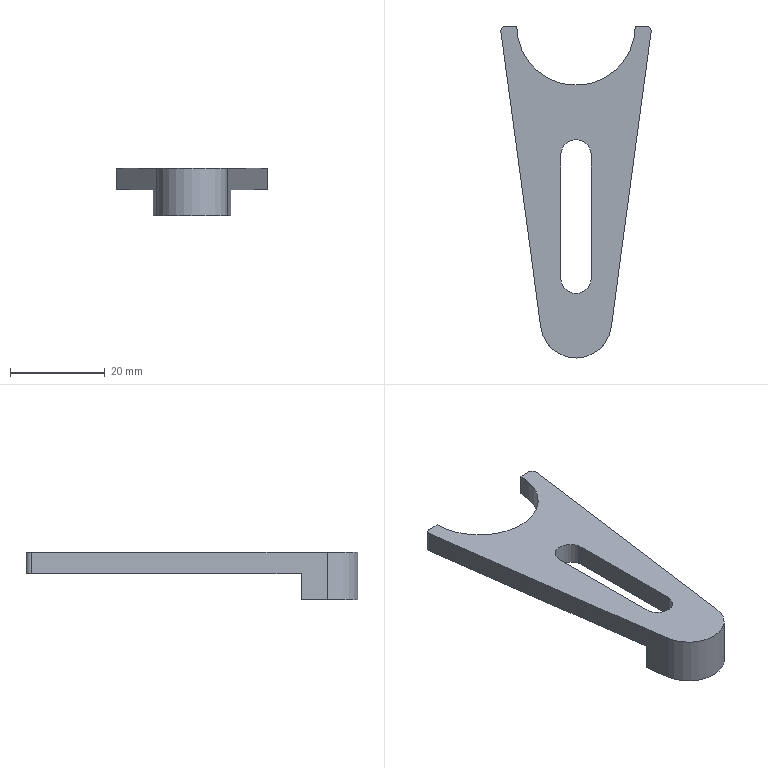Part | STEP file | 1358D2-4.stp.STEP | 1 solid | 16 faces | box 31.712 x 70 x 10 mm | volume 5901 mm3 | plane 10 | cylinder 6 | commonest cylinder face diameters 2 x2 6.4 x2 15 x1 25 x1
STEP:
#1=CARTESIAN_POINT('',(8.175,-23.,0.));
#2=VERTEX_POINT('',#1);
#3=CARTESIAN_POINT('',(7.433,-28.503,0.));
#4=VERTEX_POINT('',#3);
#5=CARTESIAN_POINT('',(8.175,-23.,0.));
#6=DIRECTION('',(-0.1337,-0.991,0.));
#7=VECTOR('',#6,1000.);
#8=LINE('',#5,#7);
#9=EDGE_CURVE('',#2,#4,#8,.T.);
#10=ORIENTED_EDGE('',*,*,#9,.T.);
#11=CARTESIAN_POINT('',(-7.433,-28.503,0.));
#12=VERTEX_POINT('',#11);
#13=CARTESIAN_POINT('',(0.,-27.5,0.));
#14=DIRECTION('',(0.,0.,1.));
#15=DIRECTION('',(-0.991,-0.1337,0.));
#16=AXIS2_PLACEMENT_3D('',#13,#14,#15);
#17=CIRCLE('',#16,7.5);
#18=EDGE_CURVE('',#12,#4,#17,.T.);
#19=ORIENTED_EDGE('',*,*,#18,.F.);
#20=CARTESIAN_POINT('',(-8.175,-23.,0.));
#21=VERTEX_POINT('',#20);
#22=CARTESIAN_POINT('',(-7.433,-28.503,0.));
#23=DIRECTION('',(-0.1337,0.991,0.));
#24=VECTOR('',#23,1000.);
#25=LINE('',#22,#24);
#26=EDGE_CURVE('',#12,#21,#25,.T.);
#27=ORIENTED_EDGE('',*,*,#26,.T.);
#28=CARTESIAN_POINT('',(-8.175,-23.,0.));
#29=DIRECTION('',(1.,0.,0.));
#30=VECTOR('',#29,1000.);
#31=LINE('',#28,#30);
#32=EDGE_CURVE('',#21,#2,#31,.T.);
#33=ORIENTED_EDGE('',*,*,#32,.T.);
#34=EDGE_LOOP('',(#10,#19,#27,#33));
#35=FACE_OUTER_BOUND('',#34,.T.);
#36=CARTESIAN_POINT('',(0.,0.,0.));
#37=DIRECTION('',(0.,0.,1.));
#38=DIRECTION('',(1.,0.,0.));
#39=AXIS2_PLACEMENT_3D('',#36,#37,#38);
#40=PLANE('',#39);
#41=ADVANCED_FACE('',(#35),#40,.F.);
#42=CARTESIAN_POINT('',(-8.175,-23.,5.5));
#43=VERTEX_POINT('',#42);
#44=CARTESIAN_POINT('',(-8.175,-23.,0.));
#45=DIRECTION('',(0.,0.,1.));
#46=VECTOR('',#45,1000.);
#47=LINE('',#44,#46);
#48=EDGE_CURVE('',#21,#43,#47,.T.);
#49=ORIENTED_EDGE('',*,*,#48,.T.);
#50=CARTESIAN_POINT('',(8.175,-23.,5.5));
#51=VERTEX_POINT('',#50);
#52=CARTESIAN_POINT('',(8.175,-23.,5.5));
#53=DIRECTION('',(-1.,0.,0.));
#54=VECTOR('',#53,1000.);
#55=LINE('',#52,#54);
#56=EDGE_CURVE('',#51,#43,#55,.T.);
#57=ORIENTED_EDGE('',*,*,#56,.F.);
#58=CARTESIAN_POINT('',(8.175,-23.,0.));
#59=DIRECTION('',(0.,0.,1.));
#60=VECTOR('',#59,1000.);
#61=LINE('',#58,#60);
#62=EDGE_CURVE('',#2,#51,#61,.T.);
#63=ORIENTED_EDGE('',*,*,#62,.F.);
#64=ORIENTED_EDGE('',*,*,#32,.F.);
#65=EDGE_LOOP('',(#49,#57,#63,#64));
#66=FACE_OUTER_BOUND('',#65,.T.);
#67=CARTESIAN_POINT('',(30.,-23.,0.));
#68=DIRECTION('',(0.,-1.,0.));
#69=DIRECTION('',(0.,0.,-1.));
#70=AXIS2_PLACEMENT_3D('',#67,#68,#69);
#71=PLANE('',#70);
#72=ADVANCED_FACE('',(#66),#71,.F.);
#73=CARTESIAN_POINT('',(15.847,33.866,10.));
#74=VERTEX_POINT('',#73);
#75=CARTESIAN_POINT('',(7.433,-28.503,10.));
#76=VERTEX_POINT('',#75);
#77=CARTESIAN_POINT('',(15.847,33.866,10.));
#78=DIRECTION('',(-0.1337,-0.991,0.));
#79=VECTOR('',#78,1000.);
#80=LINE('',#77,#79);
#81=EDGE_CURVE('',#74,#76,#80,.T.);
#82=ORIENTED_EDGE('',*,*,#81,.T.);
#83=CARTESIAN_POINT('',(7.433,-28.503,10.));
#84=DIRECTION('',(0.,0.,-1.));
#85=VECTOR('',#84,1000.);
#86=LINE('',#83,#85);
#87=EDGE_CURVE('',#76,#4,#86,.T.);
#88=ORIENTED_EDGE('',*,*,#87,.T.);
#89=ORIENTED_EDGE('',*,*,#9,.F.);
#90=ORIENTED_EDGE('',*,*,#62,.T.);
#91=CARTESIAN_POINT('',(15.847,33.866,5.5));
#92=VERTEX_POINT('',#91);
#93=CARTESIAN_POINT('',(15.847,33.866,5.5));
#94=DIRECTION('',(-0.1337,-0.991,0.));
#95=VECTOR('',#94,1000.);
#96=LINE('',#93,#95);
#97=EDGE_CURVE('',#92,#51,#96,.T.);
#98=ORIENTED_EDGE('',*,*,#97,.F.);
#99=CARTESIAN_POINT('',(15.847,33.866,10.));
#100=DIRECTION('',(0.,0.,-1.));
#101=VECTOR('',#100,1000.);
#102=LINE('',#99,#101);
#103=EDGE_CURVE('',#74,#92,#102,.T.);
#104=ORIENTED_EDGE('',*,*,#103,.F.);
#105=EDGE_LOOP('',(#82,#88,#89,#90,#98,#104));
#106=FACE_OUTER_BOUND('',#105,.T.);
#107=CARTESIAN_POINT('',(16.,35.,10.));
#108=DIRECTION('',(-0.991,0.1337,0.));
#109=DIRECTION('',(0.,0.,1.));
#110=AXIS2_PLACEMENT_3D('',#107,#108,#109);
#111=PLANE('',#110);
#112=ADVANCED_FACE('',(#106),#111,.F.);
#113=CARTESIAN_POINT('',(14.856,35.,10.));
#114=VERTEX_POINT('',#113);
#115=CARTESIAN_POINT('',(14.856,35.,5.5));
#116=VERTEX_POINT('',#115);
#117=CARTESIAN_POINT('',(14.856,35.,10.));
#118=DIRECTION('',(0.,0.,-1.));
#119=VECTOR('',#118,1000.);
#120=LINE('',#117,#119);
#121=EDGE_CURVE('',#114,#116,#120,.T.);
#122=ORIENTED_EDGE('',*,*,#121,.F.);
#123=CARTESIAN_POINT('',(14.856,34.,10.));
#124=DIRECTION('',(0.,0.,1.));
#125=DIRECTION('',(0.991,-0.1337,0.));
#126=AXIS2_PLACEMENT_3D('',#123,#124,#125);
#127=CIRCLE('',#126,1.);
#128=EDGE_CURVE('',#74,#114,#127,.T.);
#129=ORIENTED_EDGE('',*,*,#128,.F.);
#130=ORIENTED_EDGE('',*,*,#103,.T.);
#131=CARTESIAN_POINT('',(14.856,34.,5.5));
#132=DIRECTION('',(0.,0.,-1.));
#133=DIRECTION('',(0.,1.,0.));
#134=AXIS2_PLACEMENT_3D('',#131,#132,#133);
#135=CIRCLE('',#134,1.);
#136=EDGE_CURVE('',#116,#92,#135,.T.);
#137=ORIENTED_EDGE('',*,*,#136,.F.);
#138=EDGE_LOOP('',(#122,#129,#130,#137));
#139=FACE_OUTER_BOUND('',#138,.T.);
#140=CARTESIAN_POINT('',(14.856,34.,23.036));
#141=DIRECTION('',(0.,0.,-1.));
#142=DIRECTION('',(0.,1.,0.));
#143=AXIS2_PLACEMENT_3D('',#140,#141,#142);
#144=CYLINDRICAL_SURFACE('',#143,1.);
#145=ADVANCED_FACE('',(#139),#144,.T.);
#146=CARTESIAN_POINT('',(3.2,-18.2,5.5));
#147=VERTEX_POINT('',#146);
#148=CARTESIAN_POINT('',(-3.2,-18.2,5.5));
#149=VERTEX_POINT('',#148);
#150=CARTESIAN_POINT('',(0.,-18.2,5.5));
#151=DIRECTION('',(0.,0.,-1.));
#152=DIRECTION('',(1.,0.,0.));
#153=AXIS2_PLACEMENT_3D('',#150,#151,#152);
#154=CIRCLE('',#153,3.2);
#155=EDGE_CURVE('',#147,#149,#154,.T.);
#156=ORIENTED_EDGE('',*,*,#155,.F.);
#157=CARTESIAN_POINT('',(3.2,7.8,5.5));
#158=VERTEX_POINT('',#157);
#159=CARTESIAN_POINT('',(3.2,-18.2,5.5));
#160=DIRECTION('',(0.,1.,0.));
#161=VECTOR('',#160,1000.);
#162=LINE('',#159,#161);
#163=EDGE_CURVE('',#147,#158,#162,.T.);
#164=ORIENTED_EDGE('',*,*,#163,.T.);
#165=CARTESIAN_POINT('',(-3.2,7.8,5.5));
#166=VERTEX_POINT('',#165);
#167=CARTESIAN_POINT('',(0.,7.8,5.5));
#168=DIRECTION('',(0.,0.,1.));
#169=DIRECTION('',(1.,0.,0.));
#170=AXIS2_PLACEMENT_3D('',#167,#168,#169);
#171=CIRCLE('',#170,3.2);
#172=EDGE_CURVE('',#158,#166,#171,.T.);
#173=ORIENTED_EDGE('',*,*,#172,.T.);
#174=CARTESIAN_POINT('',(-3.2,7.8,5.5));
#175=DIRECTION('',(0.,-1.,0.));
#176=VECTOR('',#175,1000.);
#177=LINE('',#174,#176);
#178=EDGE_CURVE('',#166,#149,#177,.T.);
#179=ORIENTED_EDGE('',*,*,#178,.T.);
#180=EDGE_LOOP('',(#156,#164,#173,#179));
#181=FACE_BOUND('',#180,.T.);
#182=CARTESIAN_POINT('',(-12.5,35.,5.5));
#183=VERTEX_POINT('',#182);
#184=CARTESIAN_POINT('',(-14.856,35.,5.5));
#185=VERTEX_POINT('',#184);
#186=CARTESIAN_POINT('',(-12.5,35.,5.5));
#187=DIRECTION('',(-1.,0.,0.));
#188=VECTOR('',#187,1000.);
#189=LINE('',#186,#188);
#190=EDGE_CURVE('',#183,#185,#189,.T.);
#191=ORIENTED_EDGE('',*,*,#190,.F.);
#192=CARTESIAN_POINT('',(12.5,35.,5.5));
#193=VERTEX_POINT('',#192);
#194=CARTESIAN_POINT('',(0.,35.,5.5));
#195=DIRECTION('',(0.,0.,1.));
#196=DIRECTION('',(-1.,0.,0.));
#197=AXIS2_PLACEMENT_3D('',#194,#195,#196);
#198=CIRCLE('',#197,12.5);
#199=EDGE_CURVE('',#183,#193,#198,.T.);
#200=ORIENTED_EDGE('',*,*,#199,.T.);
#201=CARTESIAN_POINT('',(14.856,35.,5.5));
#202=DIRECTION('',(-1.,0.,0.));
#203=VECTOR('',#202,1000.);
#204=LINE('',#201,#203);
#205=EDGE_CURVE('',#116,#193,#204,.T.);
#206=ORIENTED_EDGE('',*,*,#205,.F.);
#207=ORIENTED_EDGE('',*,*,#136,.T.);
#208=ORIENTED_EDGE('',*,*,#97,.T.);
#209=ORIENTED_EDGE('',*,*,#56,.T.);
#210=CARTESIAN_POINT('',(-15.847,33.866,5.5));
#211=VERTEX_POINT('',#210);
#212=CARTESIAN_POINT('',(-15.847,33.866,5.5));
#213=DIRECTION('',(0.1337,-0.991,0.));
#214=VECTOR('',#213,1000.);
#215=LINE('',#212,#214);
#216=EDGE_CURVE('',#211,#43,#215,.T.);
#217=ORIENTED_EDGE('',*,*,#216,.F.);
#218=CARTESIAN_POINT('',(-14.856,34.,5.5));
#219=DIRECTION('',(0.,0.,-1.));
#220=DIRECTION('',(-0.991,-0.1337,0.));
#221=AXIS2_PLACEMENT_3D('',#218,#219,#220);
#222=CIRCLE('',#221,1.);
#223=EDGE_CURVE('',#211,#185,#222,.T.);
#224=ORIENTED_EDGE('',*,*,#223,.T.);
#225=EDGE_LOOP('',(#191,#200,#206,#207,#208,#209,#217,#224));
#226=FACE_OUTER_BOUND('',#225,.T.);
#227=CARTESIAN_POINT('',(0.,0.,5.5));
#228=DIRECTION('',(0.,0.,-1.));
#229=DIRECTION('',(0.,-1.,0.));
#230=AXIS2_PLACEMENT_3D('',#227,#228,#229);
#231=PLANE('',#230);
#232=ADVANCED_FACE('',(#181,#226),#231,.T.);
#233=CARTESIAN_POINT('',(-3.2,7.8,10.));
#234=VERTEX_POINT('',#233);
#235=CARTESIAN_POINT('',(-3.2,7.8,5.5));
#236=DIRECTION('',(0.,0.,1.));
#237=VECTOR('',#236,1000.);
#238=LINE('',#235,#237);
#239=EDGE_CURVE('',#166,#234,#238,.T.);
#240=ORIENTED_EDGE('',*,*,#239,.T.);
#241=CARTESIAN_POINT('',(-3.2,-18.2,10.));
#242=VERTEX_POINT('',#241);
#243=CARTESIAN_POINT('',(-3.2,7.8,10.));
#244=DIRECTION('',(0.,-1.,0.));
#245=VECTOR('',#244,1000.);
#246=LINE('',#243,#245);
#247=EDGE_CURVE('',#234,#242,#246,.T.);
#248=ORIENTED_EDGE('',*,*,#247,.T.);
#249=CARTESIAN_POINT('',(-3.2,-18.2,10.));
#250=DIRECTION('',(0.,0.,-1.));
#251=VECTOR('',#250,1000.);
#252=LINE('',#249,#251);
#253=EDGE_CURVE('',#242,#149,#252,.T.);
#254=ORIENTED_EDGE('',*,*,#253,.T.);
#255=ORIENTED_EDGE('',*,*,#178,.F.);
#256=EDGE_LOOP('',(#240,#248,#254,#255));
#257=FACE_OUTER_BOUND('',#256,.T.);
#258=CARTESIAN_POINT('',(-3.2,11.,10.));
#259=DIRECTION('',(-1.,0.,0.));
#260=DIRECTION('',(0.,0.,1.));
#261=AXIS2_PLACEMENT_3D('',#258,#259,#260);
#262=PLANE('',#261);
#263=ADVANCED_FACE('',(#257),#262,.F.);
#264=ORIENTED_EDGE('',*,*,#253,.F.);
#265=CARTESIAN_POINT('',(3.2,-18.2,10.));
#266=VERTEX_POINT('',#265);
#267=CARTESIAN_POINT('',(0.,-18.2,10.));
#268=DIRECTION('',(0.,0.,-1.));
#269=DIRECTION('',(1.,0.,0.));
#270=AXIS2_PLACEMENT_3D('',#267,#268,#269);
#271=CIRCLE('',#270,3.2);
#272=EDGE_CURVE('',#266,#242,#271,.T.);
#273=ORIENTED_EDGE('',*,*,#272,.F.);
#274=CARTESIAN_POINT('',(3.2,-18.2,10.));
#275=DIRECTION('',(0.,0.,-1.));
#276=VECTOR('',#275,1000.);
#277=LINE('',#274,#276);
#278=EDGE_CURVE('',#266,#147,#277,.T.);
#279=ORIENTED_EDGE('',*,*,#278,.T.);
#280=ORIENTED_EDGE('',*,*,#155,.T.);
#281=EDGE_LOOP('',(#264,#273,#279,#280));
#282=FACE_OUTER_BOUND('',#281,.T.);
#283=CARTESIAN_POINT('',(0.,-18.2,10.143));
#284=DIRECTION('',(0.,0.,-1.));
#285=DIRECTION('',(1.,0.,0.));
#286=AXIS2_PLACEMENT_3D('',#283,#284,#285);
#287=CYLINDRICAL_SURFACE('',#286,3.2);
#288=ADVANCED_FACE('',(#282),#287,.F.);
#289=ORIENTED_EDGE('',*,*,#278,.F.);
#290=CARTESIAN_POINT('',(3.2,7.8,10.));
#291=VERTEX_POINT('',#290);
#292=CARTESIAN_POINT('',(3.2,-18.2,10.));
#293=DIRECTION('',(0.,1.,0.));
#294=VECTOR('',#293,1000.);
#295=LINE('',#292,#294);
#296=EDGE_CURVE('',#266,#291,#295,.T.);
#297=ORIENTED_EDGE('',*,*,#296,.T.);
#298=CARTESIAN_POINT('',(3.2,7.8,5.5));
#299=DIRECTION('',(0.,0.,1.));
#300=VECTOR('',#299,1000.);
#301=LINE('',#298,#300);
#302=EDGE_CURVE('',#158,#291,#301,.T.);
#303=ORIENTED_EDGE('',*,*,#302,.F.);
#304=ORIENTED_EDGE('',*,*,#163,.F.);
#305=EDGE_LOOP('',(#289,#297,#303,#304));
#306=FACE_OUTER_BOUND('',#305,.T.);
#307=CARTESIAN_POINT('',(3.2,-21.4,10.));
#308=DIRECTION('',(1.,0.,0.));
#309=DIRECTION('',(0.,1.,0.));
#310=AXIS2_PLACEMENT_3D('',#307,#308,#309);
#311=PLANE('',#310);
#312=ADVANCED_FACE('',(#306),#311,.F.);
#313=ORIENTED_EDGE('',*,*,#302,.T.);
#314=CARTESIAN_POINT('',(0.,7.8,10.));
#315=DIRECTION('',(0.,0.,-1.));
#316=DIRECTION('',(-1.,0.,0.));
#317=AXIS2_PLACEMENT_3D('',#314,#315,#316);
#318=CIRCLE('',#317,3.2);
#319=EDGE_CURVE('',#234,#291,#318,.T.);
#320=ORIENTED_EDGE('',*,*,#319,.F.);
#321=ORIENTED_EDGE('',*,*,#239,.F.);
#322=ORIENTED_EDGE('',*,*,#172,.F.);
#323=EDGE_LOOP('',(#313,#320,#321,#322));
#324=FACE_OUTER_BOUND('',#323,.T.);
#325=CARTESIAN_POINT('',(0.,7.8,-0.1224));
#326=DIRECTION('',(0.,0.,1.));
#327=DIRECTION('',(1.,0.,0.));
#328=AXIS2_PLACEMENT_3D('',#325,#326,#327);
#329=CYLINDRICAL_SURFACE('',#328,3.2);
#330=ADVANCED_FACE('',(#324),#329,.F.);
#331=ORIENTED_EDGE('',*,*,#319,.T.);
#332=ORIENTED_EDGE('',*,*,#296,.F.);
#333=ORIENTED_EDGE('',*,*,#272,.T.);
#334=ORIENTED_EDGE('',*,*,#247,.F.);
#335=EDGE_LOOP('',(#331,#332,#333,#334));
#336=FACE_BOUND('',#335,.T.);
#337=CARTESIAN_POINT('',(-7.433,-28.503,10.));
#338=VERTEX_POINT('',#337);
#339=CARTESIAN_POINT('',(-15.847,33.866,10.));
#340=VERTEX_POINT('',#339);
#341=CARTESIAN_POINT('',(-7.433,-28.503,10.));
#342=DIRECTION('',(-0.1337,0.991,0.));
#343=VECTOR('',#342,1000.);
#344=LINE('',#341,#343);
#345=EDGE_CURVE('',#338,#340,#344,.T.);
#346=ORIENTED_EDGE('',*,*,#345,.F.);
#347=CARTESIAN_POINT('',(0.,-27.5,10.));
#348=DIRECTION('',(0.,0.,-1.));
#349=DIRECTION('',(0.991,-0.1337,0.));
#350=AXIS2_PLACEMENT_3D('',#347,#348,#349);
#351=CIRCLE('',#350,7.5);
#352=EDGE_CURVE('',#76,#338,#351,.T.);
#353=ORIENTED_EDGE('',*,*,#352,.F.);
#354=ORIENTED_EDGE('',*,*,#81,.F.);
#355=ORIENTED_EDGE('',*,*,#128,.T.);
#356=CARTESIAN_POINT('',(12.5,35.,10.));
#357=VERTEX_POINT('',#356);
#358=CARTESIAN_POINT('',(14.856,35.,10.));
#359=DIRECTION('',(-1.,0.,0.));
#360=VECTOR('',#359,1000.);
#361=LINE('',#358,#360);
#362=EDGE_CURVE('',#114,#357,#361,.T.);
#363=ORIENTED_EDGE('',*,*,#362,.T.);
#364=CARTESIAN_POINT('',(-12.5,35.,10.));
#365=VERTEX_POINT('',#364);
#366=CARTESIAN_POINT('',(0.,35.,10.));
#367=DIRECTION('',(0.,0.,1.));
#368=DIRECTION('',(-1.,0.,0.));
#369=AXIS2_PLACEMENT_3D('',#366,#367,#368);
#370=CIRCLE('',#369,12.5);
#371=EDGE_CURVE('',#365,#357,#370,.T.);
#372=ORIENTED_EDGE('',*,*,#371,.F.);
#373=CARTESIAN_POINT('',(-14.856,35.,10.));
#374=VERTEX_POINT('',#373);
#375=CARTESIAN_POINT('',(-12.5,35.,10.));
#376=DIRECTION('',(-1.,0.,0.));
#377=VECTOR('',#376,1000.);
#378=LINE('',#375,#377);
#379=EDGE_CURVE('',#365,#374,#378,.T.);
#380=ORIENTED_EDGE('',*,*,#379,.T.);
#381=CARTESIAN_POINT('',(-14.856,34.,10.));
#382=DIRECTION('',(0.,0.,1.));
#383=DIRECTION('',(0.,1.,0.));
#384=AXIS2_PLACEMENT_3D('',#381,#382,#383);
#385=CIRCLE('',#384,1.);
#386=EDGE_CURVE('',#374,#340,#385,.T.);
#387=ORIENTED_EDGE('',*,*,#386,.T.);
#388=EDGE_LOOP('',(#346,#353,#354,#355,#363,#372,#380,#387));
#389=FACE_OUTER_BOUND('',#388,.T.);
#390=CARTESIAN_POINT('',(0.,0.,10.));
#391=DIRECTION('',(0.,0.,1.));
#392=DIRECTION('',(1.,0.,0.));
#393=AXIS2_PLACEMENT_3D('',#390,#391,#392);
#394=PLANE('',#393);
#395=ADVANCED_FACE('',(#336,#389),#394,.T.);
#396=CARTESIAN_POINT('',(-14.856,35.,5.5));
#397=DIRECTION('',(0.,0.,1.));
#398=VECTOR('',#397,1000.);
#399=LINE('',#396,#398);
#400=EDGE_CURVE('',#185,#374,#399,.T.);
#401=ORIENTED_EDGE('',*,*,#400,.F.);
#402=ORIENTED_EDGE('',*,*,#223,.F.);
#403=CARTESIAN_POINT('',(-15.847,33.866,5.5));
#404=DIRECTION('',(0.,0.,1.));
#405=VECTOR('',#404,1000.);
#406=LINE('',#403,#405);
#407=EDGE_CURVE('',#211,#340,#406,.T.);
#408=ORIENTED_EDGE('',*,*,#407,.T.);
#409=ORIENTED_EDGE('',*,*,#386,.F.);
#410=EDGE_LOOP('',(#401,#402,#408,#409));
#411=FACE_OUTER_BOUND('',#410,.T.);
#412=CARTESIAN_POINT('',(-14.856,34.,-13.036));
#413=DIRECTION('',(0.,0.,1.));
#414=DIRECTION('',(0.,1.,0.));
#415=AXIS2_PLACEMENT_3D('',#412,#413,#414);
#416=CYLINDRICAL_SURFACE('',#415,1.);
#417=ADVANCED_FACE('',(#411),#416,.T.);
#418=ORIENTED_EDGE('',*,*,#216,.T.);
#419=ORIENTED_EDGE('',*,*,#48,.F.);
#420=ORIENTED_EDGE('',*,*,#26,.F.);
#421=CARTESIAN_POINT('',(-7.433,-28.503,10.));
#422=DIRECTION('',(0.,0.,-1.));
#423=VECTOR('',#422,1000.);
#424=LINE('',#421,#423);
#425=EDGE_CURVE('',#338,#12,#424,.T.);
#426=ORIENTED_EDGE('',*,*,#425,.F.);
#427=ORIENTED_EDGE('',*,*,#345,.T.);
#428=ORIENTED_EDGE('',*,*,#407,.F.);
#429=EDGE_LOOP('',(#418,#419,#420,#426,#427,#428));
#430=FACE_OUTER_BOUND('',#429,.T.);
#431=CARTESIAN_POINT('',(-7.433,-28.503,10.));
#432=DIRECTION('',(0.991,0.1337,0.));
#433=DIRECTION('',(0.,0.,-1.));
#434=AXIS2_PLACEMENT_3D('',#431,#432,#433);
#435=PLANE('',#434);
#436=ADVANCED_FACE('',(#430),#435,.F.);
#437=ORIENTED_EDGE('',*,*,#87,.F.);
#438=ORIENTED_EDGE('',*,*,#352,.T.);
#439=ORIENTED_EDGE('',*,*,#425,.T.);
#440=ORIENTED_EDGE('',*,*,#18,.T.);
#441=EDGE_LOOP('',(#437,#438,#439,#440));
#442=FACE_OUTER_BOUND('',#441,.T.);
#443=CARTESIAN_POINT('',(0.,-27.5,10.));
#444=DIRECTION('',(0.,0.,1.));
#445=DIRECTION('',(1.,0.,0.));
#446=AXIS2_PLACEMENT_3D('',#443,#444,#445);
#447=CYLINDRICAL_SURFACE('',#446,7.5);
#448=ADVANCED_FACE('',(#442),#447,.T.);
#449=ORIENTED_EDGE('',*,*,#379,.F.);
#450=CARTESIAN_POINT('',(-12.5,35.,5.5));
#451=DIRECTION('',(0.,0.,1.));
#452=VECTOR('',#451,1000.);
#453=LINE('',#450,#452);
#454=EDGE_CURVE('',#183,#365,#453,.T.);
#455=ORIENTED_EDGE('',*,*,#454,.F.);
#456=ORIENTED_EDGE('',*,*,#190,.T.);
#457=ORIENTED_EDGE('',*,*,#400,.T.);
#458=EDGE_LOOP('',(#449,#455,#456,#457));
#459=FACE_OUTER_BOUND('',#458,.T.);
#460=CARTESIAN_POINT('',(22.5,35.,0.));
#461=DIRECTION('',(0.,1.,0.));
#462=DIRECTION('',(1.,0.,0.));
#463=AXIS2_PLACEMENT_3D('',#460,#461,#462);
#464=PLANE('',#463);
#465=ADVANCED_FACE('',(#459),#464,.T.);
#466=ORIENTED_EDGE('',*,*,#205,.T.);
#467=CARTESIAN_POINT('',(12.5,35.,5.5));
#468=DIRECTION('',(0.,0.,1.));
#469=VECTOR('',#468,1000.);
#470=LINE('',#467,#469);
#471=EDGE_CURVE('',#193,#357,#470,.T.);
#472=ORIENTED_EDGE('',*,*,#471,.T.);
#473=ORIENTED_EDGE('',*,*,#362,.F.);
#474=ORIENTED_EDGE('',*,*,#121,.T.);
#475=EDGE_LOOP('',(#466,#472,#473,#474));
#476=FACE_OUTER_BOUND('',#475,.T.);
#477=CARTESIAN_POINT('',(22.5,35.,0.));
#478=DIRECTION('',(0.,1.,0.));
#479=DIRECTION('',(1.,0.,0.));
#480=AXIS2_PLACEMENT_3D('',#477,#478,#479);
#481=PLANE('',#480);
#482=ADVANCED_FACE('',(#476),#481,.T.);
#483=ORIENTED_EDGE('',*,*,#454,.T.);
#484=ORIENTED_EDGE('',*,*,#371,.T.);
#485=ORIENTED_EDGE('',*,*,#471,.F.);
#486=ORIENTED_EDGE('',*,*,#199,.F.);
#487=EDGE_LOOP('',(#483,#484,#485,#486));
#488=FACE_OUTER_BOUND('',#487,.T.);
#489=CARTESIAN_POINT('',(0.,35.,10.));
#490=DIRECTION('',(0.,0.,1.));
#491=DIRECTION('',(1.,0.,0.));
#492=AXIS2_PLACEMENT_3D('',#489,#490,#491);
#493=CYLINDRICAL_SURFACE('',#492,12.5);
#494=ADVANCED_FACE('',(#488),#493,.F.);
#495=CLOSED_SHELL('',(#41,#72,#112,#145,#232,#263,#288,#312,#330,#395,#417,#436,#448,#465,#482,#494));
#496=MANIFOLD_SOLID_BREP('',#495);
#497=CARTESIAN_POINT('',(0.,0.,0.));
#498=DIRECTION('',(0.,0.,1.));
#499=DIRECTION('',(1.,0.,0.));
#500=AXIS2_PLACEMENT_3D('',#497,#498,#499);
#501=(LENGTH_UNIT()NAMED_UNIT(*)SI_UNIT(.MILLI.,.METRE.));
#502=UNCERTAINTY_MEASURE_WITH_UNIT(LENGTH_MEASURE(0.00001),#501,'','');
#503=(NAMED_UNIT(*)PLANE_ANGLE_UNIT()SI_UNIT($,.RADIAN.));
#504=(NAMED_UNIT(*)SI_UNIT($,.STERADIAN.)SOLID_ANGLE_UNIT());
#505=(GEOMETRIC_REPRESENTATION_CONTEXT(3)GLOBAL_UNCERTAINTY_ASSIGNED_CONTEXT((#502))GLOBAL_UNIT_ASSIGNED_CONTEXT((#501,#503,#504))REPRESENTATION_CONTEXT('',''));
#506=ADVANCED_BREP_SHAPE_REPRESENTATION('',(#496,#500),#505);